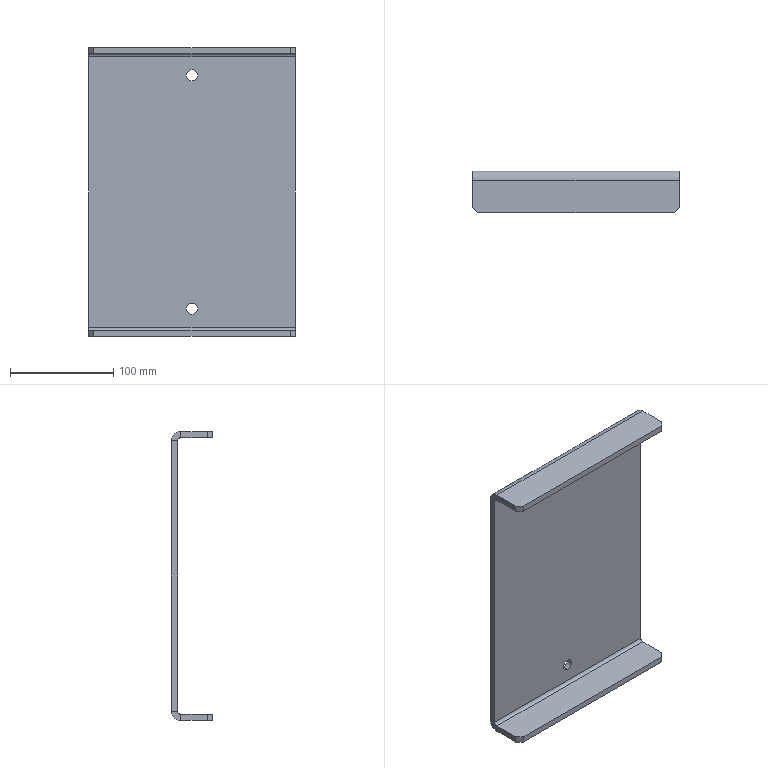Part | STEP file | 100 | 1 solid | 30 faces | box 200 x 40 x 280 mm | volume 410020 mm3 | plane 22 | cylinder 8 | commonest cylinder face diameters 10.8 x4 6 x2 18 x2
STEP:
#1=CARTESIAN_POINT('',(-95.,-40.,134.));
#2=VERTEX_POINT('',#1);
#3=CARTESIAN_POINT('',(-95.,-40.,140.));
#4=VERTEX_POINT('',#3);
#5=CARTESIAN_POINT('',(-95.,-40.,134.));
#6=DIRECTION('',(0.,0.,1.));
#7=VECTOR('',#6,1000.);
#8=LINE('',#5,#7);
#9=EDGE_CURVE('',#2,#4,#8,.T.);
#10=ORIENTED_EDGE('',*,*,#9,.T.);
#11=CARTESIAN_POINT('',(-100.,-35.,140.));
#12=VERTEX_POINT('',#11);
#13=CARTESIAN_POINT('',(-100.,-35.,140.));
#14=DIRECTION('',(0.7071,-0.7071,0.));
#15=VECTOR('',#14,1000.);
#16=LINE('',#13,#15);
#17=EDGE_CURVE('',#12,#4,#16,.T.);
#18=ORIENTED_EDGE('',*,*,#17,.F.);
#19=CARTESIAN_POINT('',(-100.,-35.,134.));
#20=VERTEX_POINT('',#19);
#21=CARTESIAN_POINT('',(-100.,-35.,140.));
#22=DIRECTION('',(0.,0.,-1.));
#23=VECTOR('',#22,1000.);
#24=LINE('',#21,#23);
#25=EDGE_CURVE('',#12,#20,#24,.T.);
#26=ORIENTED_EDGE('',*,*,#25,.T.);
#27=CARTESIAN_POINT('',(-95.,-40.,134.));
#28=DIRECTION('',(-0.7071,0.7071,0.));
#29=VECTOR('',#28,1000.);
#30=LINE('',#27,#29);
#31=EDGE_CURVE('',#2,#20,#30,.T.);
#32=ORIENTED_EDGE('',*,*,#31,.F.);
#33=EDGE_LOOP('',(#10,#18,#26,#32));
#34=FACE_OUTER_BOUND('',#33,.T.);
#35=CARTESIAN_POINT('',(-100.,-35.,131.));
#36=DIRECTION('',(0.7071,0.7071,0.));
#37=DIRECTION('',(0.,0.,-1.));
#38=AXIS2_PLACEMENT_3D('',#35,#36,#37);
#39=PLANE('',#38);
#40=ADVANCED_FACE('',(#34),#39,.F.);
#41=CARTESIAN_POINT('',(-100.,-9.,140.));
#42=VERTEX_POINT('',#41);
#43=CARTESIAN_POINT('',(100.,-9.,140.));
#44=VERTEX_POINT('',#43);
#45=CARTESIAN_POINT('',(-100.,-9.,140.));
#46=DIRECTION('',(1.,0.,0.));
#47=VECTOR('',#46,1000.);
#48=LINE('',#45,#47);
#49=EDGE_CURVE('',#42,#44,#48,.T.);
#50=ORIENTED_EDGE('',*,*,#49,.T.);
#51=CARTESIAN_POINT('',(100.,0.,131.));
#52=VERTEX_POINT('',#51);
#53=CARTESIAN_POINT('',(100.,-9.,131.));
#54=DIRECTION('',(1.,0.,0.));
#55=DIRECTION('',(0.,1.,0.));
#56=AXIS2_PLACEMENT_3D('',#53,#54,#55);
#57=CIRCLE('',#56,9.);
#58=EDGE_CURVE('',#52,#44,#57,.T.);
#59=ORIENTED_EDGE('',*,*,#58,.F.);
#60=CARTESIAN_POINT('',(-100.,0.,131.));
#61=VERTEX_POINT('',#60);
#62=CARTESIAN_POINT('',(100.,0.,131.));
#63=DIRECTION('',(-1.,0.,0.));
#64=VECTOR('',#63,1000.);
#65=LINE('',#62,#64);
#66=EDGE_CURVE('',#52,#61,#65,.T.);
#67=ORIENTED_EDGE('',*,*,#66,.T.);
#68=CARTESIAN_POINT('',(-100.,-9.,131.));
#69=DIRECTION('',(-1.,0.,0.));
#70=DIRECTION('',(0.,0.,1.));
#71=AXIS2_PLACEMENT_3D('',#68,#69,#70);
#72=CIRCLE('',#71,9.);
#73=EDGE_CURVE('',#42,#61,#72,.T.);
#74=ORIENTED_EDGE('',*,*,#73,.F.);
#75=EDGE_LOOP('',(#50,#59,#67,#74));
#76=FACE_OUTER_BOUND('',#75,.T.);
#77=CARTESIAN_POINT('',(100.,-9.,131.));
#78=DIRECTION('',(-1.,0.,0.));
#79=DIRECTION('',(0.,0.,1.));
#80=AXIS2_PLACEMENT_3D('',#77,#78,#79);
#81=CYLINDRICAL_SURFACE('',#80,9.);
#82=ADVANCED_FACE('',(#76),#81,.T.);
#83=CARTESIAN_POINT('',(0.,-6.,-107.6));
#84=VERTEX_POINT('',#83);
#85=CARTESIAN_POINT('',(0.,-6.,-118.4));
#86=VERTEX_POINT('',#85);
#87=CARTESIAN_POINT('',(0.,-6.,-113.));
#88=DIRECTION('',(0.,1.,0.));
#89=DIRECTION('',(0.,0.,1.));
#90=AXIS2_PLACEMENT_3D('',#87,#88,#89);
#91=CIRCLE('',#90,5.4);
#92=EDGE_CURVE('',#84,#86,#91,.T.);
#93=ORIENTED_EDGE('',*,*,#92,.F.);
#94=CARTESIAN_POINT('',(0.,0.,-107.6));
#95=VERTEX_POINT('',#94);
#96=CARTESIAN_POINT('',(0.,0.,-107.6));
#97=DIRECTION('',(0.,-1.,0.));
#98=VECTOR('',#97,1000.);
#99=LINE('',#96,#98);
#100=EDGE_CURVE('',#95,#84,#99,.T.);
#101=ORIENTED_EDGE('',*,*,#100,.F.);
#102=CARTESIAN_POINT('',(0.,0.,-118.4));
#103=VERTEX_POINT('',#102);
#104=CARTESIAN_POINT('',(0.,0.,-113.));
#105=DIRECTION('',(0.,-1.,0.));
#106=DIRECTION('',(0.,0.,-1.));
#107=AXIS2_PLACEMENT_3D('',#104,#105,#106);
#108=CIRCLE('',#107,5.4);
#109=EDGE_CURVE('',#103,#95,#108,.T.);
#110=ORIENTED_EDGE('',*,*,#109,.F.);
#111=CARTESIAN_POINT('',(0.,0.,-118.4));
#112=DIRECTION('',(0.,-1.,0.));
#113=VECTOR('',#112,1000.);
#114=LINE('',#111,#113);
#115=EDGE_CURVE('',#103,#86,#114,.T.);
#116=ORIENTED_EDGE('',*,*,#115,.T.);
#117=EDGE_LOOP('',(#93,#101,#110,#116));
#118=FACE_OUTER_BOUND('',#117,.T.);
#119=CARTESIAN_POINT('',(0.,-10.,-113.));
#120=DIRECTION('',(0.,1.,0.));
#121=DIRECTION('',(0.,0.,1.));
#122=AXIS2_PLACEMENT_3D('',#119,#120,#121);
#123=CYLINDRICAL_SURFACE('',#122,5.4);
#124=ADVANCED_FACE('',(#118),#123,.F.);
#125=ORIENTED_EDGE('',*,*,#115,.F.);
#126=CARTESIAN_POINT('',(0.,0.,-113.));
#127=DIRECTION('',(0.,-1.,0.));
#128=DIRECTION('',(0.,0.,1.));
#129=AXIS2_PLACEMENT_3D('',#126,#127,#128);
#130=CIRCLE('',#129,5.4);
#131=EDGE_CURVE('',#95,#103,#130,.T.);
#132=ORIENTED_EDGE('',*,*,#131,.F.);
#133=ORIENTED_EDGE('',*,*,#100,.T.);
#134=CARTESIAN_POINT('',(0.,-6.,-113.));
#135=DIRECTION('',(0.,1.,0.));
#136=DIRECTION('',(0.,0.,-1.));
#137=AXIS2_PLACEMENT_3D('',#134,#135,#136);
#138=CIRCLE('',#137,5.4);
#139=EDGE_CURVE('',#86,#84,#138,.T.);
#140=ORIENTED_EDGE('',*,*,#139,.F.);
#141=EDGE_LOOP('',(#125,#132,#133,#140));
#142=FACE_OUTER_BOUND('',#141,.T.);
#143=CARTESIAN_POINT('',(0.,-10.,-113.));
#144=DIRECTION('',(0.,1.,0.));
#145=DIRECTION('',(0.,0.,1.));
#146=AXIS2_PLACEMENT_3D('',#143,#144,#145);
#147=CYLINDRICAL_SURFACE('',#146,5.4);
#148=ADVANCED_FACE('',(#142),#147,.F.);
#149=CARTESIAN_POINT('',(0.,-6.,118.4));
#150=VERTEX_POINT('',#149);
#151=CARTESIAN_POINT('',(0.,-6.,107.6));
#152=VERTEX_POINT('',#151);
#153=CARTESIAN_POINT('',(0.,-6.,113.));
#154=DIRECTION('',(0.,1.,0.));
#155=DIRECTION('',(0.,0.,1.));
#156=AXIS2_PLACEMENT_3D('',#153,#154,#155);
#157=CIRCLE('',#156,5.4);
#158=EDGE_CURVE('',#150,#152,#157,.T.);
#159=ORIENTED_EDGE('',*,*,#158,.F.);
#160=CARTESIAN_POINT('',(0.,0.,118.4));
#161=VERTEX_POINT('',#160);
#162=CARTESIAN_POINT('',(0.,0.,118.4));
#163=DIRECTION('',(0.,-1.,0.));
#164=VECTOR('',#163,1000.);
#165=LINE('',#162,#164);
#166=EDGE_CURVE('',#161,#150,#165,.T.);
#167=ORIENTED_EDGE('',*,*,#166,.F.);
#168=CARTESIAN_POINT('',(0.,0.,107.6));
#169=VERTEX_POINT('',#168);
#170=CARTESIAN_POINT('',(0.,0.,113.));
#171=DIRECTION('',(0.,-1.,0.));
#172=DIRECTION('',(0.,0.,-1.));
#173=AXIS2_PLACEMENT_3D('',#170,#171,#172);
#174=CIRCLE('',#173,5.4);
#175=EDGE_CURVE('',#169,#161,#174,.T.);
#176=ORIENTED_EDGE('',*,*,#175,.F.);
#177=CARTESIAN_POINT('',(0.,0.,107.6));
#178=DIRECTION('',(0.,-1.,0.));
#179=VECTOR('',#178,1000.);
#180=LINE('',#177,#179);
#181=EDGE_CURVE('',#169,#152,#180,.T.);
#182=ORIENTED_EDGE('',*,*,#181,.T.);
#183=EDGE_LOOP('',(#159,#167,#176,#182));
#184=FACE_OUTER_BOUND('',#183,.T.);
#185=CARTESIAN_POINT('',(0.,-10.,113.));
#186=DIRECTION('',(0.,1.,0.));
#187=DIRECTION('',(0.,0.,1.));
#188=AXIS2_PLACEMENT_3D('',#185,#186,#187);
#189=CYLINDRICAL_SURFACE('',#188,5.4);
#190=ADVANCED_FACE('',(#184),#189,.F.);
#191=ORIENTED_EDGE('',*,*,#181,.F.);
#192=CARTESIAN_POINT('',(0.,0.,113.));
#193=DIRECTION('',(0.,-1.,0.));
#194=DIRECTION('',(0.,0.,1.));
#195=AXIS2_PLACEMENT_3D('',#192,#193,#194);
#196=CIRCLE('',#195,5.4);
#197=EDGE_CURVE('',#161,#169,#196,.T.);
#198=ORIENTED_EDGE('',*,*,#197,.F.);
#199=ORIENTED_EDGE('',*,*,#166,.T.);
#200=CARTESIAN_POINT('',(0.,-6.,113.));
#201=DIRECTION('',(0.,1.,0.));
#202=DIRECTION('',(0.,0.,-1.));
#203=AXIS2_PLACEMENT_3D('',#200,#201,#202);
#204=CIRCLE('',#203,5.4);
#205=EDGE_CURVE('',#152,#150,#204,.T.);
#206=ORIENTED_EDGE('',*,*,#205,.F.);
#207=EDGE_LOOP('',(#191,#198,#199,#206));
#208=FACE_OUTER_BOUND('',#207,.T.);
#209=CARTESIAN_POINT('',(0.,-10.,113.));
#210=DIRECTION('',(0.,1.,0.));
#211=DIRECTION('',(0.,0.,1.));
#212=AXIS2_PLACEMENT_3D('',#209,#210,#211);
#213=CYLINDRICAL_SURFACE('',#212,5.4);
#214=ADVANCED_FACE('',(#208),#213,.F.);
#215=CARTESIAN_POINT('',(-100.,0.,-131.));
#216=VERTEX_POINT('',#215);
#217=CARTESIAN_POINT('',(100.,0.,-131.));
#218=VERTEX_POINT('',#217);
#219=CARTESIAN_POINT('',(-100.,0.,-131.));
#220=DIRECTION('',(1.,0.,0.));
#221=VECTOR('',#220,1000.);
#222=LINE('',#219,#221);
#223=EDGE_CURVE('',#216,#218,#222,.T.);
#224=ORIENTED_EDGE('',*,*,#223,.T.);
#225=CARTESIAN_POINT('',(100.,-9.,-140.));
#226=VERTEX_POINT('',#225);
#227=CARTESIAN_POINT('',(100.,-9.,-131.));
#228=DIRECTION('',(1.,0.,0.));
#229=DIRECTION('',(0.,0.,-1.));
#230=AXIS2_PLACEMENT_3D('',#227,#228,#229);
#231=CIRCLE('',#230,9.);
#232=EDGE_CURVE('',#226,#218,#231,.T.);
#233=ORIENTED_EDGE('',*,*,#232,.F.);
#234=CARTESIAN_POINT('',(-100.,-9.,-140.));
#235=VERTEX_POINT('',#234);
#236=CARTESIAN_POINT('',(100.,-9.,-140.));
#237=DIRECTION('',(-1.,0.,0.));
#238=VECTOR('',#237,1000.);
#239=LINE('',#236,#238);
#240=EDGE_CURVE('',#226,#235,#239,.T.);
#241=ORIENTED_EDGE('',*,*,#240,.T.);
#242=CARTESIAN_POINT('',(-100.,-9.,-131.));
#243=DIRECTION('',(-1.,0.,0.));
#244=DIRECTION('',(0.,1.,0.));
#245=AXIS2_PLACEMENT_3D('',#242,#243,#244);
#246=CIRCLE('',#245,9.);
#247=EDGE_CURVE('',#216,#235,#246,.T.);
#248=ORIENTED_EDGE('',*,*,#247,.F.);
#249=EDGE_LOOP('',(#224,#233,#241,#248));
#250=FACE_OUTER_BOUND('',#249,.T.);
#251=CARTESIAN_POINT('',(100.,-9.,-131.));
#252=DIRECTION('',(-1.,0.,0.));
#253=DIRECTION('',(0.,0.,1.));
#254=AXIS2_PLACEMENT_3D('',#251,#252,#253);
#255=CYLINDRICAL_SURFACE('',#254,9.);
#256=ADVANCED_FACE('',(#250),#255,.T.);
#257=ORIENTED_EDGE('',*,*,#232,.T.);
#258=CARTESIAN_POINT('',(100.,-6.,-131.));
#259=VERTEX_POINT('',#258);
#260=CARTESIAN_POINT('',(100.,0.,-131.));
#261=DIRECTION('',(0.,-1.,0.));
#262=VECTOR('',#261,1000.);
#263=LINE('',#260,#262);
#264=EDGE_CURVE('',#218,#259,#263,.T.);
#265=ORIENTED_EDGE('',*,*,#264,.T.);
#266=CARTESIAN_POINT('',(100.,-9.,-134.));
#267=VERTEX_POINT('',#266);
#268=CARTESIAN_POINT('',(100.,-9.,-131.));
#269=DIRECTION('',(-1.,0.,0.));
#270=DIRECTION('',(0.,1.,0.));
#271=AXIS2_PLACEMENT_3D('',#268,#269,#270);
#272=CIRCLE('',#271,3.);
#273=EDGE_CURVE('',#259,#267,#272,.T.);
#274=ORIENTED_EDGE('',*,*,#273,.T.);
#275=CARTESIAN_POINT('',(100.,-9.,-134.));
#276=DIRECTION('',(0.,0.,-1.));
#277=VECTOR('',#276,1000.);
#278=LINE('',#275,#277);
#279=EDGE_CURVE('',#267,#226,#278,.T.);
#280=ORIENTED_EDGE('',*,*,#279,.T.);
#281=EDGE_LOOP('',(#257,#265,#274,#280));
#282=FACE_OUTER_BOUND('',#281,.T.);
#283=CARTESIAN_POINT('',(100.,-9.,-140.));
#284=DIRECTION('',(1.,0.,0.));
#285=DIRECTION('',(0.,1.,0.));
#286=AXIS2_PLACEMENT_3D('',#283,#284,#285);
#287=PLANE('',#286);
#288=ADVANCED_FACE('',(#282),#287,.T.);
#289=CARTESIAN_POINT('',(100.,-35.,-140.));
#290=VERTEX_POINT('',#289);
#291=CARTESIAN_POINT('',(100.,-35.,-134.));
#292=VERTEX_POINT('',#291);
#293=CARTESIAN_POINT('',(100.,-35.,-140.));
#294=DIRECTION('',(0.,0.,1.));
#295=VECTOR('',#294,1000.);
#296=LINE('',#293,#295);
#297=EDGE_CURVE('',#290,#292,#296,.T.);
#298=ORIENTED_EDGE('',*,*,#297,.T.);
#299=CARTESIAN_POINT('',(95.,-40.,-134.));
#300=VERTEX_POINT('',#299);
#301=CARTESIAN_POINT('',(95.,-40.,-134.));
#302=DIRECTION('',(0.7071,0.7071,0.));
#303=VECTOR('',#302,1000.);
#304=LINE('',#301,#303);
#305=EDGE_CURVE('',#300,#292,#304,.T.);
#306=ORIENTED_EDGE('',*,*,#305,.F.);
#307=CARTESIAN_POINT('',(95.,-40.,-140.));
#308=VERTEX_POINT('',#307);
#309=CARTESIAN_POINT('',(95.,-40.,-134.));
#310=DIRECTION('',(0.,0.,-1.));
#311=VECTOR('',#310,1000.);
#312=LINE('',#309,#311);
#313=EDGE_CURVE('',#300,#308,#312,.T.);
#314=ORIENTED_EDGE('',*,*,#313,.T.);
#315=CARTESIAN_POINT('',(100.,-35.,-140.));
#316=DIRECTION('',(-0.7071,-0.7071,0.));
#317=VECTOR('',#316,1000.);
#318=LINE('',#315,#317);
#319=EDGE_CURVE('',#290,#308,#318,.T.);
#320=ORIENTED_EDGE('',*,*,#319,.F.);
#321=EDGE_LOOP('',(#298,#306,#314,#320));
#322=FACE_OUTER_BOUND('',#321,.T.);
#323=CARTESIAN_POINT('',(95.,-40.,-140.));
#324=DIRECTION('',(-0.7071,0.7071,0.));
#325=DIRECTION('',(0.,0.,1.));
#326=AXIS2_PLACEMENT_3D('',#323,#324,#325);
#327=PLANE('',#326);
#328=ADVANCED_FACE('',(#322),#327,.F.);
#329=CARTESIAN_POINT('',(-95.,-40.,-140.));
#330=VERTEX_POINT('',#329);
#331=CARTESIAN_POINT('',(-95.,-40.,-134.));
#332=VERTEX_POINT('',#331);
#333=CARTESIAN_POINT('',(-95.,-40.,-140.));
#334=DIRECTION('',(0.,0.,1.));
#335=VECTOR('',#334,1000.);
#336=LINE('',#333,#335);
#337=EDGE_CURVE('',#330,#332,#336,.T.);
#338=ORIENTED_EDGE('',*,*,#337,.T.);
#339=CARTESIAN_POINT('',(-100.,-35.,-134.));
#340=VERTEX_POINT('',#339);
#341=CARTESIAN_POINT('',(-100.,-35.,-134.));
#342=DIRECTION('',(0.7071,-0.7071,0.));
#343=VECTOR('',#342,1000.);
#344=LINE('',#341,#343);
#345=EDGE_CURVE('',#340,#332,#344,.T.);
#346=ORIENTED_EDGE('',*,*,#345,.F.);
#347=CARTESIAN_POINT('',(-100.,-35.,-140.));
#348=VERTEX_POINT('',#347);
#349=CARTESIAN_POINT('',(-100.,-35.,-134.));
#350=DIRECTION('',(0.,0.,-1.));
#351=VECTOR('',#350,1000.);
#352=LINE('',#349,#351);
#353=EDGE_CURVE('',#340,#348,#352,.T.);
#354=ORIENTED_EDGE('',*,*,#353,.T.);
#355=CARTESIAN_POINT('',(-95.,-40.,-140.));
#356=DIRECTION('',(-0.7071,0.7071,0.));
#357=VECTOR('',#356,1000.);
#358=LINE('',#355,#357);
#359=EDGE_CURVE('',#330,#348,#358,.T.);
#360=ORIENTED_EDGE('',*,*,#359,.F.);
#361=EDGE_LOOP('',(#338,#346,#354,#360));
#362=FACE_OUTER_BOUND('',#361,.T.);
#363=CARTESIAN_POINT('',(-100.,-35.,131.));
#364=DIRECTION('',(-0.7071,-0.7071,0.));
#365=DIRECTION('',(-0.7071,0.7071,0.));
#366=AXIS2_PLACEMENT_3D('',#363,#364,#365);
#367=PLANE('',#366);
#368=ADVANCED_FACE('',(#362),#367,.T.);
#369=ORIENTED_EDGE('',*,*,#313,.F.);
#370=CARTESIAN_POINT('',(-95.,-40.,-134.));
#371=DIRECTION('',(1.,0.,0.));
#372=VECTOR('',#371,1000.);
#373=LINE('',#370,#372);
#374=EDGE_CURVE('',#332,#300,#373,.T.);
#375=ORIENTED_EDGE('',*,*,#374,.F.);
#376=ORIENTED_EDGE('',*,*,#337,.F.);
#377=CARTESIAN_POINT('',(-95.,-40.,-140.));
#378=DIRECTION('',(1.,0.,0.));
#379=VECTOR('',#378,1000.);
#380=LINE('',#377,#379);
#381=EDGE_CURVE('',#330,#308,#380,.T.);
#382=ORIENTED_EDGE('',*,*,#381,.T.);
#383=EDGE_LOOP('',(#369,#375,#376,#382));
#384=FACE_OUTER_BOUND('',#383,.T.);
#385=CARTESIAN_POINT('',(100.,-40.,-140.));
#386=DIRECTION('',(0.,-1.,0.));
#387=DIRECTION('',(0.,0.,-1.));
#388=AXIS2_PLACEMENT_3D('',#385,#386,#387);
#389=PLANE('',#388);
#390=ADVANCED_FACE('',(#384),#389,.T.);
#391=ORIENTED_EDGE('',*,*,#305,.T.);
#392=CARTESIAN_POINT('',(100.,-9.,-134.));
#393=DIRECTION('',(0.,-1.,0.));
#394=VECTOR('',#393,1000.);
#395=LINE('',#392,#394);
#396=EDGE_CURVE('',#267,#292,#395,.T.);
#397=ORIENTED_EDGE('',*,*,#396,.F.);
#398=CARTESIAN_POINT('',(-100.,-9.,-134.));
#399=VERTEX_POINT('',#398);
#400=CARTESIAN_POINT('',(-100.,-9.,-134.));
#401=DIRECTION('',(1.,0.,0.));
#402=VECTOR('',#401,1000.);
#403=LINE('',#400,#402);
#404=EDGE_CURVE('',#399,#267,#403,.T.);
#405=ORIENTED_EDGE('',*,*,#404,.F.);
#406=CARTESIAN_POINT('',(-100.,-9.,-134.));
#407=DIRECTION('',(0.,-1.,0.));
#408=VECTOR('',#407,1000.);
#409=LINE('',#406,#408);
#410=EDGE_CURVE('',#399,#340,#409,.T.);
#411=ORIENTED_EDGE('',*,*,#410,.T.);
#412=ORIENTED_EDGE('',*,*,#345,.T.);
#413=ORIENTED_EDGE('',*,*,#374,.T.);
#414=EDGE_LOOP('',(#391,#397,#405,#411,#412,#413));
#415=FACE_OUTER_BOUND('',#414,.T.);
#416=CARTESIAN_POINT('',(100.,0.,-134.));
#417=DIRECTION('',(0.,0.,1.));
#418=DIRECTION('',(1.,0.,0.));
#419=AXIS2_PLACEMENT_3D('',#416,#417,#418);
#420=PLANE('',#419);
#421=ADVANCED_FACE('',(#415),#420,.T.);
#422=ORIENTED_EDGE('',*,*,#297,.F.);
#423=CARTESIAN_POINT('',(100.,-9.,-140.));
#424=DIRECTION('',(0.,-1.,0.));
#425=VECTOR('',#424,1000.);
#426=LINE('',#423,#425);
#427=EDGE_CURVE('',#226,#290,#426,.T.);
#428=ORIENTED_EDGE('',*,*,#427,.F.);
#429=ORIENTED_EDGE('',*,*,#279,.F.);
#430=ORIENTED_EDGE('',*,*,#396,.T.);
#431=EDGE_LOOP('',(#422,#428,#429,#430));
#432=FACE_OUTER_BOUND('',#431,.T.);
#433=CARTESIAN_POINT('',(100.,-6.,-131.));
#434=DIRECTION('',(1.,0.,0.));
#435=DIRECTION('',(0.,1.,0.));
#436=AXIS2_PLACEMENT_3D('',#433,#434,#435);
#437=PLANE('',#436);
#438=ADVANCED_FACE('',(#432),#437,.T.);
#439=ORIENTED_EDGE('',*,*,#319,.T.);
#440=ORIENTED_EDGE('',*,*,#381,.F.);
#441=ORIENTED_EDGE('',*,*,#359,.T.);
#442=CARTESIAN_POINT('',(-100.,-9.,-140.));
#443=DIRECTION('',(0.,-1.,0.));
#444=VECTOR('',#443,1000.);
#445=LINE('',#442,#444);
#446=EDGE_CURVE('',#235,#348,#445,.T.);
#447=ORIENTED_EDGE('',*,*,#446,.F.);
#448=ORIENTED_EDGE('',*,*,#240,.F.);
#449=ORIENTED_EDGE('',*,*,#427,.T.);
#450=EDGE_LOOP('',(#439,#440,#441,#447,#448,#449));
#451=FACE_OUTER_BOUND('',#450,.T.);
#452=CARTESIAN_POINT('',(100.,0.,-140.));
#453=DIRECTION('',(0.,0.,1.));
#454=DIRECTION('',(1.,0.,0.));
#455=AXIS2_PLACEMENT_3D('',#452,#453,#454);
#456=PLANE('',#455);
#457=ADVANCED_FACE('',(#451),#456,.F.);
#458=ORIENTED_EDGE('',*,*,#353,.F.);
#459=ORIENTED_EDGE('',*,*,#410,.F.);
#460=CARTESIAN_POINT('',(-100.,-9.,-140.));
#461=DIRECTION('',(0.,0.,1.));
#462=VECTOR('',#461,1000.);
#463=LINE('',#460,#462);
#464=EDGE_CURVE('',#235,#399,#463,.T.);
#465=ORIENTED_EDGE('',*,*,#464,.F.);
#466=ORIENTED_EDGE('',*,*,#446,.T.);
#467=EDGE_LOOP('',(#458,#459,#465,#466));
#468=FACE_OUTER_BOUND('',#467,.T.);
#469=CARTESIAN_POINT('',(-100.,-9.,131.));
#470=DIRECTION('',(1.,0.,0.));
#471=DIRECTION('',(0.,1.,0.));
#472=AXIS2_PLACEMENT_3D('',#469,#470,#471);
#473=PLANE('',#472);
#474=ADVANCED_FACE('',(#468),#473,.F.);
#475=ORIENTED_EDGE('',*,*,#247,.T.);
#476=ORIENTED_EDGE('',*,*,#464,.T.);
#477=CARTESIAN_POINT('',(-100.,-6.,-131.));
#478=VERTEX_POINT('',#477);
#479=CARTESIAN_POINT('',(-100.,-9.,-131.));
#480=DIRECTION('',(1.,0.,0.));
#481=DIRECTION('',(0.,0.,-1.));
#482=AXIS2_PLACEMENT_3D('',#479,#480,#481);
#483=CIRCLE('',#482,3.);
#484=EDGE_CURVE('',#399,#478,#483,.T.);
#485=ORIENTED_EDGE('',*,*,#484,.T.);
#486=CARTESIAN_POINT('',(-100.,-6.,-131.));
#487=DIRECTION('',(0.,1.,0.));
#488=VECTOR('',#487,1000.);
#489=LINE('',#486,#488);
#490=EDGE_CURVE('',#478,#216,#489,.T.);
#491=ORIENTED_EDGE('',*,*,#490,.T.);
#492=EDGE_LOOP('',(#475,#476,#485,#491));
#493=FACE_OUTER_BOUND('',#492,.T.);
#494=CARTESIAN_POINT('',(-100.,0.,-131.));
#495=DIRECTION('',(-1.,0.,0.));
#496=DIRECTION('',(0.,0.,1.));
#497=AXIS2_PLACEMENT_3D('',#494,#495,#496);
#498=PLANE('',#497);
#499=ADVANCED_FACE('',(#493),#498,.T.);
#500=ORIENTED_EDGE('',*,*,#404,.T.);
#501=ORIENTED_EDGE('',*,*,#273,.F.);
#502=CARTESIAN_POINT('',(100.,-6.,-131.));
#503=DIRECTION('',(-1.,0.,0.));
#504=VECTOR('',#503,1000.);
#505=LINE('',#502,#504);
#506=EDGE_CURVE('',#259,#478,#505,.T.);
#507=ORIENTED_EDGE('',*,*,#506,.T.);
#508=ORIENTED_EDGE('',*,*,#484,.F.);
#509=EDGE_LOOP('',(#500,#501,#507,#508));
#510=FACE_OUTER_BOUND('',#509,.T.);
#511=CARTESIAN_POINT('',(100.,-9.,-131.));
#512=DIRECTION('',(-1.,0.,0.));
#513=DIRECTION('',(0.,0.,1.));
#514=AXIS2_PLACEMENT_3D('',#511,#512,#513);
#515=CYLINDRICAL_SURFACE('',#514,3.);
#516=ADVANCED_FACE('',(#510),#515,.F.);
#517=ORIENTED_EDGE('',*,*,#92,.T.);
#518=ORIENTED_EDGE('',*,*,#139,.T.);
#519=EDGE_LOOP('',(#517,#518));
#520=FACE_BOUND('',#519,.T.);
#521=ORIENTED_EDGE('',*,*,#158,.T.);
#522=ORIENTED_EDGE('',*,*,#205,.T.);
#523=EDGE_LOOP('',(#521,#522));
#524=FACE_BOUND('',#523,.T.);
#525=ORIENTED_EDGE('',*,*,#506,.F.);
#526=CARTESIAN_POINT('',(100.,-6.,131.));
#527=VERTEX_POINT('',#526);
#528=CARTESIAN_POINT('',(100.,-6.,131.));
#529=DIRECTION('',(0.,0.,-1.));
#530=VECTOR('',#529,1000.);
#531=LINE('',#528,#530);
#532=EDGE_CURVE('',#527,#259,#531,.T.);
#533=ORIENTED_EDGE('',*,*,#532,.F.);
#534=CARTESIAN_POINT('',(-100.,-6.,131.));
#535=VERTEX_POINT('',#534);
#536=CARTESIAN_POINT('',(-100.,-6.,131.));
#537=DIRECTION('',(1.,0.,0.));
#538=VECTOR('',#537,1000.);
#539=LINE('',#536,#538);
#540=EDGE_CURVE('',#535,#527,#539,.T.);
#541=ORIENTED_EDGE('',*,*,#540,.F.);
#542=CARTESIAN_POINT('',(-100.,-6.,131.));
#543=DIRECTION('',(0.,0.,-1.));
#544=VECTOR('',#543,1000.);
#545=LINE('',#542,#544);
#546=EDGE_CURVE('',#535,#478,#545,.T.);
#547=ORIENTED_EDGE('',*,*,#546,.T.);
#548=EDGE_LOOP('',(#525,#533,#541,#547));
#549=FACE_OUTER_BOUND('',#548,.T.);
#550=CARTESIAN_POINT('',(100.,-6.,140.));
#551=DIRECTION('',(0.,-1.,0.));
#552=DIRECTION('',(0.,0.,-1.));
#553=AXIS2_PLACEMENT_3D('',#550,#551,#552);
#554=PLANE('',#553);
#555=ADVANCED_FACE('',(#520,#524,#549),#554,.T.);
#556=ORIENTED_EDGE('',*,*,#540,.T.);
#557=CARTESIAN_POINT('',(100.,-9.,134.));
#558=VERTEX_POINT('',#557);
#559=CARTESIAN_POINT('',(100.,-9.,131.));
#560=DIRECTION('',(-1.,0.,0.));
#561=DIRECTION('',(0.,0.,1.));
#562=AXIS2_PLACEMENT_3D('',#559,#560,#561);
#563=CIRCLE('',#562,3.);
#564=EDGE_CURVE('',#558,#527,#563,.T.);
#565=ORIENTED_EDGE('',*,*,#564,.F.);
#566=CARTESIAN_POINT('',(-100.,-9.,134.));
#567=VERTEX_POINT('',#566);
#568=CARTESIAN_POINT('',(100.,-9.,134.));
#569=DIRECTION('',(-1.,0.,0.));
#570=VECTOR('',#569,1000.);
#571=LINE('',#568,#570);
#572=EDGE_CURVE('',#558,#567,#571,.T.);
#573=ORIENTED_EDGE('',*,*,#572,.T.);
#574=CARTESIAN_POINT('',(-100.,-9.,131.));
#575=DIRECTION('',(1.,0.,0.));
#576=DIRECTION('',(0.,1.,0.));
#577=AXIS2_PLACEMENT_3D('',#574,#575,#576);
#578=CIRCLE('',#577,3.);
#579=EDGE_CURVE('',#535,#567,#578,.T.);
#580=ORIENTED_EDGE('',*,*,#579,.F.);
#581=EDGE_LOOP('',(#556,#565,#573,#580));
#582=FACE_OUTER_BOUND('',#581,.T.);
#583=CARTESIAN_POINT('',(100.,-9.,131.));
#584=DIRECTION('',(-1.,0.,0.));
#585=DIRECTION('',(0.,0.,1.));
#586=AXIS2_PLACEMENT_3D('',#583,#584,#585);
#587=CYLINDRICAL_SURFACE('',#586,3.);
#588=ADVANCED_FACE('',(#582),#587,.F.);
#589=ORIENTED_EDGE('',*,*,#73,.T.);
#590=CARTESIAN_POINT('',(-100.,0.,131.));
#591=DIRECTION('',(0.,-1.,0.));
#592=VECTOR('',#591,1000.);
#593=LINE('',#590,#592);
#594=EDGE_CURVE('',#61,#535,#593,.T.);
#595=ORIENTED_EDGE('',*,*,#594,.T.);
#596=ORIENTED_EDGE('',*,*,#579,.T.);
#597=CARTESIAN_POINT('',(-100.,-9.,134.));
#598=DIRECTION('',(0.,0.,1.));
#599=VECTOR('',#598,1000.);
#600=LINE('',#597,#599);
#601=EDGE_CURVE('',#567,#42,#600,.T.);
#602=ORIENTED_EDGE('',*,*,#601,.T.);
#603=EDGE_LOOP('',(#589,#595,#596,#602));
#604=FACE_OUTER_BOUND('',#603,.T.);
#605=CARTESIAN_POINT('',(-100.,-9.,140.));
#606=DIRECTION('',(-1.,0.,0.));
#607=DIRECTION('',(0.,0.,1.));
#608=AXIS2_PLACEMENT_3D('',#605,#606,#607);
#609=PLANE('',#608);
#610=ADVANCED_FACE('',(#604),#609,.T.);
#611=ORIENTED_EDGE('',*,*,#490,.F.);
#612=ORIENTED_EDGE('',*,*,#546,.F.);
#613=ORIENTED_EDGE('',*,*,#594,.F.);
#614=CARTESIAN_POINT('',(-100.,0.,131.));
#615=DIRECTION('',(0.,0.,-1.));
#616=VECTOR('',#615,1000.);
#617=LINE('',#614,#616);
#618=EDGE_CURVE('',#61,#216,#617,.T.);
#619=ORIENTED_EDGE('',*,*,#618,.T.);
#620=EDGE_LOOP('',(#611,#612,#613,#619));
#621=FACE_OUTER_BOUND('',#620,.T.);
#622=CARTESIAN_POINT('',(-100.,-9.,-134.));
#623=DIRECTION('',(-1.,0.,0.));
#624=DIRECTION('',(0.,0.,1.));
#625=AXIS2_PLACEMENT_3D('',#622,#623,#624);
#626=PLANE('',#625);
#627=ADVANCED_FACE('',(#621),#626,.T.);
#628=ORIENTED_EDGE('',*,*,#131,.T.);
#629=ORIENTED_EDGE('',*,*,#109,.T.);
#630=EDGE_LOOP('',(#628,#629));
#631=FACE_BOUND('',#630,.T.);
#632=ORIENTED_EDGE('',*,*,#197,.T.);
#633=ORIENTED_EDGE('',*,*,#175,.T.);
#634=EDGE_LOOP('',(#632,#633));
#635=FACE_BOUND('',#634,.T.);
#636=ORIENTED_EDGE('',*,*,#66,.F.);
#637=CARTESIAN_POINT('',(100.,0.,131.));
#638=DIRECTION('',(0.,0.,-1.));
#639=VECTOR('',#638,1000.);
#640=LINE('',#637,#639);
#641=EDGE_CURVE('',#52,#218,#640,.T.);
#642=ORIENTED_EDGE('',*,*,#641,.T.);
#643=ORIENTED_EDGE('',*,*,#223,.F.);
#644=ORIENTED_EDGE('',*,*,#618,.F.);
#645=EDGE_LOOP('',(#636,#642,#643,#644));
#646=FACE_OUTER_BOUND('',#645,.T.);
#647=CARTESIAN_POINT('',(100.,0.,140.));
#648=DIRECTION('',(0.,-1.,0.));
#649=DIRECTION('',(0.,0.,-1.));
#650=AXIS2_PLACEMENT_3D('',#647,#648,#649);
#651=PLANE('',#650);
#652=ADVANCED_FACE('',(#631,#635,#646),#651,.F.);
#653=CARTESIAN_POINT('',(100.,-6.,131.));
#654=DIRECTION('',(0.,1.,0.));
#655=VECTOR('',#654,1000.);
#656=LINE('',#653,#655);
#657=EDGE_CURVE('',#527,#52,#656,.T.);
#658=ORIENTED_EDGE('',*,*,#657,.F.);
#659=ORIENTED_EDGE('',*,*,#532,.T.);
#660=ORIENTED_EDGE('',*,*,#264,.F.);
#661=ORIENTED_EDGE('',*,*,#641,.F.);
#662=EDGE_LOOP('',(#658,#659,#660,#661));
#663=FACE_OUTER_BOUND('',#662,.T.);
#664=CARTESIAN_POINT('',(100.,-9.,134.));
#665=DIRECTION('',(1.,0.,0.));
#666=DIRECTION('',(0.,1.,0.));
#667=AXIS2_PLACEMENT_3D('',#664,#665,#666);
#668=PLANE('',#667);
#669=ADVANCED_FACE('',(#663),#668,.T.);
#670=ORIENTED_EDGE('',*,*,#58,.T.);
#671=CARTESIAN_POINT('',(100.,-9.,140.));
#672=DIRECTION('',(0.,0.,-1.));
#673=VECTOR('',#672,1000.);
#674=LINE('',#671,#673);
#675=EDGE_CURVE('',#44,#558,#674,.T.);
#676=ORIENTED_EDGE('',*,*,#675,.T.);
#677=ORIENTED_EDGE('',*,*,#564,.T.);
#678=ORIENTED_EDGE('',*,*,#657,.T.);
#679=EDGE_LOOP('',(#670,#676,#677,#678));
#680=FACE_OUTER_BOUND('',#679,.T.);
#681=CARTESIAN_POINT('',(100.,0.,131.));
#682=DIRECTION('',(1.,0.,0.));
#683=DIRECTION('',(0.,1.,0.));
#684=AXIS2_PLACEMENT_3D('',#681,#682,#683);
#685=PLANE('',#684);
#686=ADVANCED_FACE('',(#680),#685,.T.);
#687=CARTESIAN_POINT('',(100.,-35.,134.));
#688=VERTEX_POINT('',#687);
#689=CARTESIAN_POINT('',(100.,-35.,140.));
#690=VERTEX_POINT('',#689);
#691=CARTESIAN_POINT('',(100.,-35.,134.));
#692=DIRECTION('',(0.,0.,1.));
#693=VECTOR('',#692,1000.);
#694=LINE('',#691,#693);
#695=EDGE_CURVE('',#688,#690,#694,.T.);
#696=ORIENTED_EDGE('',*,*,#695,.F.);
#697=CARTESIAN_POINT('',(100.,-35.,134.));
#698=DIRECTION('',(0.,1.,0.));
#699=VECTOR('',#698,1000.);
#700=LINE('',#697,#699);
#701=EDGE_CURVE('',#688,#558,#700,.T.);
#702=ORIENTED_EDGE('',*,*,#701,.T.);
#703=ORIENTED_EDGE('',*,*,#675,.F.);
#704=CARTESIAN_POINT('',(100.,-35.,140.));
#705=DIRECTION('',(0.,1.,0.));
#706=VECTOR('',#705,1000.);
#707=LINE('',#704,#706);
#708=EDGE_CURVE('',#690,#44,#707,.T.);
#709=ORIENTED_EDGE('',*,*,#708,.F.);
#710=EDGE_LOOP('',(#696,#702,#703,#709));
#711=FACE_OUTER_BOUND('',#710,.T.);
#712=CARTESIAN_POINT('',(100.,-9.,131.));
#713=DIRECTION('',(1.,0.,0.));
#714=DIRECTION('',(0.,1.,0.));
#715=AXIS2_PLACEMENT_3D('',#712,#713,#714);
#716=PLANE('',#715);
#717=ADVANCED_FACE('',(#711),#716,.T.);
#718=ORIENTED_EDGE('',*,*,#695,.T.);
#719=CARTESIAN_POINT('',(95.,-40.,140.));
#720=VERTEX_POINT('',#719);
#721=CARTESIAN_POINT('',(95.,-40.,140.));
#722=DIRECTION('',(0.7071,0.7071,0.));
#723=VECTOR('',#722,1000.);
#724=LINE('',#721,#723);
#725=EDGE_CURVE('',#720,#690,#724,.T.);
#726=ORIENTED_EDGE('',*,*,#725,.F.);
#727=CARTESIAN_POINT('',(95.,-40.,134.));
#728=VERTEX_POINT('',#727);
#729=CARTESIAN_POINT('',(95.,-40.,140.));
#730=DIRECTION('',(0.,0.,-1.));
#731=VECTOR('',#730,1000.);
#732=LINE('',#729,#731);
#733=EDGE_CURVE('',#720,#728,#732,.T.);
#734=ORIENTED_EDGE('',*,*,#733,.T.);
#735=CARTESIAN_POINT('',(100.,-35.,134.));
#736=DIRECTION('',(-0.7071,-0.7071,0.));
#737=VECTOR('',#736,1000.);
#738=LINE('',#735,#737);
#739=EDGE_CURVE('',#688,#728,#738,.T.);
#740=ORIENTED_EDGE('',*,*,#739,.F.);
#741=EDGE_LOOP('',(#718,#726,#734,#740));
#742=FACE_OUTER_BOUND('',#741,.T.);
#743=CARTESIAN_POINT('',(95.,-40.,134.));
#744=DIRECTION('',(-0.7071,0.7071,0.));
#745=DIRECTION('',(0.,0.,1.));
#746=AXIS2_PLACEMENT_3D('',#743,#744,#745);
#747=PLANE('',#746);
#748=ADVANCED_FACE('',(#742),#747,.F.);
#749=ORIENTED_EDGE('',*,*,#9,.F.);
#750=CARTESIAN_POINT('',(-95.,-40.,134.));
#751=DIRECTION('',(1.,0.,0.));
#752=VECTOR('',#751,1000.);
#753=LINE('',#750,#752);
#754=EDGE_CURVE('',#2,#728,#753,.T.);
#755=ORIENTED_EDGE('',*,*,#754,.T.);
#756=ORIENTED_EDGE('',*,*,#733,.F.);
#757=CARTESIAN_POINT('',(-95.,-40.,140.));
#758=DIRECTION('',(1.,0.,0.));
#759=VECTOR('',#758,1000.);
#760=LINE('',#757,#759);
#761=EDGE_CURVE('',#4,#720,#760,.T.);
#762=ORIENTED_EDGE('',*,*,#761,.F.);
#763=EDGE_LOOP('',(#749,#755,#756,#762));
#764=FACE_OUTER_BOUND('',#763,.T.);
#765=CARTESIAN_POINT('',(100.,-40.,134.));
#766=DIRECTION('',(0.,-1.,0.));
#767=DIRECTION('',(0.,0.,-1.));
#768=AXIS2_PLACEMENT_3D('',#765,#766,#767);
#769=PLANE('',#768);
#770=ADVANCED_FACE('',(#764),#769,.T.);
#771=ORIENTED_EDGE('',*,*,#31,.T.);
#772=CARTESIAN_POINT('',(-100.,-35.,134.));
#773=DIRECTION('',(0.,1.,0.));
#774=VECTOR('',#773,1000.);
#775=LINE('',#772,#774);
#776=EDGE_CURVE('',#20,#567,#775,.T.);
#777=ORIENTED_EDGE('',*,*,#776,.T.);
#778=ORIENTED_EDGE('',*,*,#572,.F.);
#779=ORIENTED_EDGE('',*,*,#701,.F.);
#780=ORIENTED_EDGE('',*,*,#739,.T.);
#781=ORIENTED_EDGE('',*,*,#754,.F.);
#782=EDGE_LOOP('',(#771,#777,#778,#779,#780,#781));
#783=FACE_OUTER_BOUND('',#782,.T.);
#784=CARTESIAN_POINT('',(100.,0.,134.));
#785=DIRECTION('',(0.,0.,-1.));
#786=DIRECTION('',(0.,-1.,0.));
#787=AXIS2_PLACEMENT_3D('',#784,#785,#786);
#788=PLANE('',#787);
#789=ADVANCED_FACE('',(#783),#788,.T.);
#790=ORIENTED_EDGE('',*,*,#25,.F.);
#791=CARTESIAN_POINT('',(-100.,-35.,140.));
#792=DIRECTION('',(0.,1.,0.));
#793=VECTOR('',#792,1000.);
#794=LINE('',#791,#793);
#795=EDGE_CURVE('',#12,#42,#794,.T.);
#796=ORIENTED_EDGE('',*,*,#795,.T.);
#797=ORIENTED_EDGE('',*,*,#601,.F.);
#798=ORIENTED_EDGE('',*,*,#776,.F.);
#799=EDGE_LOOP('',(#790,#796,#797,#798));
#800=FACE_OUTER_BOUND('',#799,.T.);
#801=CARTESIAN_POINT('',(-100.,-6.,131.));
#802=DIRECTION('',(-1.,0.,0.));
#803=DIRECTION('',(0.,0.,1.));
#804=AXIS2_PLACEMENT_3D('',#801,#802,#803);
#805=PLANE('',#804);
#806=ADVANCED_FACE('',(#800),#805,.T.);
#807=ORIENTED_EDGE('',*,*,#17,.T.);
#808=ORIENTED_EDGE('',*,*,#761,.T.);
#809=ORIENTED_EDGE('',*,*,#725,.T.);
#810=ORIENTED_EDGE('',*,*,#708,.T.);
#811=ORIENTED_EDGE('',*,*,#49,.F.);
#812=ORIENTED_EDGE('',*,*,#795,.F.);
#813=EDGE_LOOP('',(#807,#808,#809,#810,#811,#812));
#814=FACE_OUTER_BOUND('',#813,.T.);
#815=CARTESIAN_POINT('',(100.,0.,140.));
#816=DIRECTION('',(0.,0.,-1.));
#817=DIRECTION('',(0.,-1.,0.));
#818=AXIS2_PLACEMENT_3D('',#815,#816,#817);
#819=PLANE('',#818);
#820=ADVANCED_FACE('',(#814),#819,.F.);
#821=CLOSED_SHELL('',(#40,#82,#124,#148,#190,#214,#256,#288,#328,#368,#390,#421,#438,#457,#474,#499,#516,#555,#588,#610,#627,#652,#669,#686,#717,#748,#770,#789,#806,#820));
#822=MANIFOLD_SOLID_BREP('',#821);
#823=CARTESIAN_POINT('',(0.,0.,0.));
#824=DIRECTION('',(0.,0.,1.));
#825=DIRECTION('',(1.,0.,0.));
#826=AXIS2_PLACEMENT_3D('',#823,#824,#825);
#827=(LENGTH_UNIT()NAMED_UNIT(*)SI_UNIT(.MILLI.,.METRE.));
#828=UNCERTAINTY_MEASURE_WITH_UNIT(LENGTH_MEASURE(0.00001),#827,'','');
#829=(NAMED_UNIT(*)PLANE_ANGLE_UNIT()SI_UNIT($,.RADIAN.));
#830=(NAMED_UNIT(*)SI_UNIT($,.STERADIAN.)SOLID_ANGLE_UNIT());
#831=(GEOMETRIC_REPRESENTATION_CONTEXT(3)GLOBAL_UNCERTAINTY_ASSIGNED_CONTEXT((#828))GLOBAL_UNIT_ASSIGNED_CONTEXT((#827,#829,#830))REPRESENTATION_CONTEXT('',''));
#832=ADVANCED_BREP_SHAPE_REPRESENTATION('',(#822,#826),#831);